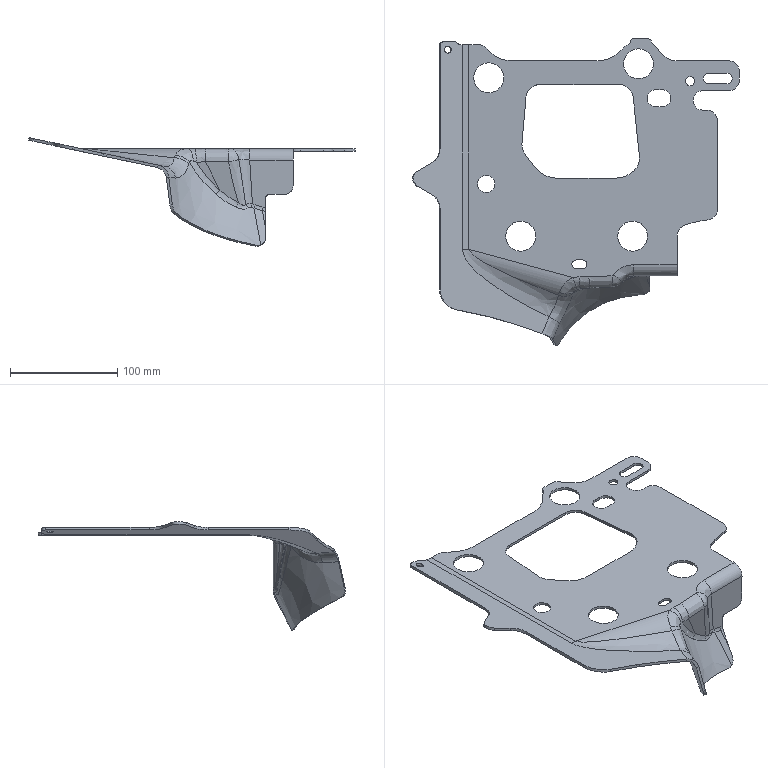Part | STEP file | K8D2-17C931-A-INS-01_id22_x_t | 1 solid | 153 faces | box 305 x 286.852 x 101.506 mm | volume 138048 mm3 | spline 83 | cylinder 44 | plane 26 | commonest cylinder face diameters 20 x6 8 x5 16 x4 28 x4 30 x3 50 x3